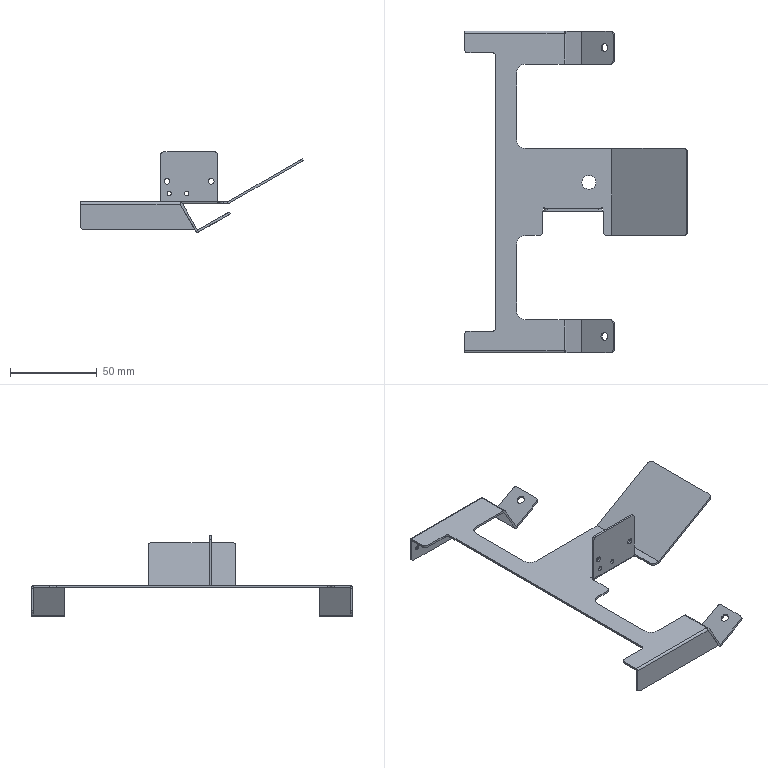Part | STEP file | unloading flow plate | 1 solid | 128 faces | box 128.223 x 185 x 46.263 mm | volume 15132 mm3 | plane 74 | cylinder 52 | spline 2 | commonest cylinder face diameters 4 x16 2.5 x14 0.1 x8 3.2 x4 4.5 x4 10 x4